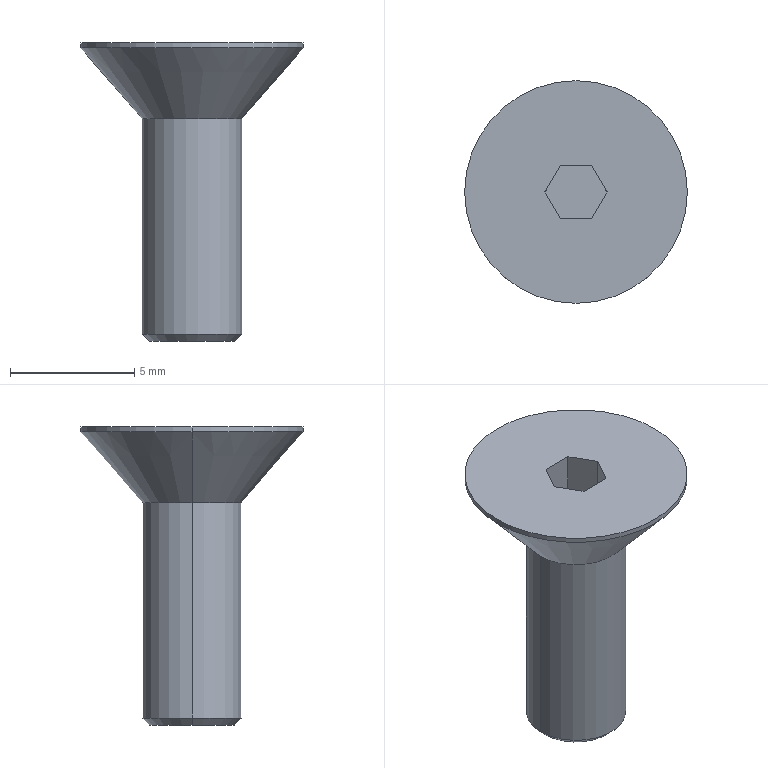Part | STEP file | 4-20.sldasm-Part-284 | 1 solid | 17 faces | box 8.96 x 8.96 x 12 mm | volume 213.091 mm3 | plane 9 | cone 4 | cylinder 4 | commonest cylinder face diameters 4 x2 8.96 x2
STEP:
#1=CARTESIAN_POINT('',(1.716,545.,-147.5));
#2=VERTEX_POINT('',#1);
#3=CARTESIAN_POINT('',(-1.716,545.,-147.5));
#4=VERTEX_POINT('',#3);
#5=CARTESIAN_POINT('',(0.,545.,-147.5));
#6=DIRECTION('',(0.,0.,-1.));
#7=DIRECTION('',(1.,0.,0.));
#8=AXIS2_PLACEMENT_3D('',#5,#6,#7);
#9=CIRCLE('',#8,1.716);
#10=EDGE_CURVE('',#2,#4,#9,.T.);
#11=ORIENTED_EDGE('',*,*,#10,.F.);
#12=CARTESIAN_POINT('',(2.,545.,-147.216));
#13=VERTEX_POINT('',#12);
#14=CARTESIAN_POINT('',(2.,545.,-147.216));
#15=DIRECTION('',(0.7071,0.,0.7071));
#16=VECTOR('',#15,1000.);
#17=LINE('',#14,#16);
#18=EDGE_CURVE('',#2,#13,#17,.T.);
#19=ORIENTED_EDGE('',*,*,#18,.T.);
#20=CARTESIAN_POINT('',(-2.,545.,-147.216));
#21=VERTEX_POINT('',#20);
#22=CARTESIAN_POINT('',(0.,545.,-147.216));
#23=DIRECTION('',(0.,0.,1.));
#24=DIRECTION('',(1.,0.,0.));
#25=AXIS2_PLACEMENT_3D('',#22,#23,#24);
#26=CIRCLE('',#25,2.);
#27=EDGE_CURVE('',#21,#13,#26,.T.);
#28=ORIENTED_EDGE('',*,*,#27,.F.);
#29=CARTESIAN_POINT('',(-2.,545.,-147.216));
#30=DIRECTION('',(-0.7071,0.,0.7071));
#31=VECTOR('',#30,1000.);
#32=LINE('',#29,#31);
#33=EDGE_CURVE('',#4,#21,#32,.T.);
#34=ORIENTED_EDGE('',*,*,#33,.F.);
#35=EDGE_LOOP('',(#11,#19,#28,#34));
#36=FACE_OUTER_BOUND('',#35,.T.);
#37=CARTESIAN_POINT('',(0.,545.,-147.216));
#38=DIRECTION('',(0.,0.,1.));
#39=DIRECTION('',(-1.,0.,0.));
#40=AXIS2_PLACEMENT_3D('',#37,#38,#39);
#41=CONICAL_SURFACE('',#40,2.,0.7854);
#42=ADVANCED_FACE('',(#36),#41,.T.);
#43=ORIENTED_EDGE('',*,*,#27,.T.);
#44=CARTESIAN_POINT('',(2.,545.,-138.553));
#45=VERTEX_POINT('',#44);
#46=CARTESIAN_POINT('',(2.,545.,-135.));
#47=DIRECTION('',(0.,0.,1.));
#48=VECTOR('',#47,1000.);
#49=LINE('',#46,#48);
#50=EDGE_CURVE('',#13,#45,#49,.T.);
#51=ORIENTED_EDGE('',*,*,#50,.T.);
#52=CARTESIAN_POINT('',(-2.,545.,-138.553));
#53=VERTEX_POINT('',#52);
#54=CARTESIAN_POINT('',(0.,545.,-138.553));
#55=DIRECTION('',(0.,0.,1.));
#56=DIRECTION('',(-1.,0.,0.));
#57=AXIS2_PLACEMENT_3D('',#54,#55,#56);
#58=CIRCLE('',#57,2.);
#59=EDGE_CURVE('',#53,#45,#58,.T.);
#60=ORIENTED_EDGE('',*,*,#59,.F.);
#61=CARTESIAN_POINT('',(-2.,545.,-135.));
#62=DIRECTION('',(0.,0.,1.));
#63=VECTOR('',#62,1000.);
#64=LINE('',#61,#63);
#65=EDGE_CURVE('',#21,#53,#64,.T.);
#66=ORIENTED_EDGE('',*,*,#65,.F.);
#67=EDGE_LOOP('',(#43,#51,#60,#66));
#68=FACE_OUTER_BOUND('',#67,.T.);
#69=CARTESIAN_POINT('',(0.,545.,-135.));
#70=DIRECTION('',(0.,0.,1.));
#71=DIRECTION('',(-1.,0.,0.));
#72=AXIS2_PLACEMENT_3D('',#69,#70,#71);
#73=CYLINDRICAL_SURFACE('',#72,2.);
#74=ADVANCED_FACE('',(#68),#73,.T.);
#75=ORIENTED_EDGE('',*,*,#59,.T.);
#76=CARTESIAN_POINT('',(4.48,545.,-135.7));
#77=VERTEX_POINT('',#76);
#78=CARTESIAN_POINT('',(4.48,545.,-135.7));
#79=DIRECTION('',(0.6561,0.,0.7547));
#80=VECTOR('',#79,1000.);
#81=LINE('',#78,#80);
#82=EDGE_CURVE('',#45,#77,#81,.T.);
#83=ORIENTED_EDGE('',*,*,#82,.T.);
#84=CARTESIAN_POINT('',(-4.48,545.,-135.7));
#85=VERTEX_POINT('',#84);
#86=CARTESIAN_POINT('',(0.,545.,-135.7));
#87=DIRECTION('',(0.,0.,1.));
#88=DIRECTION('',(-1.,0.,0.));
#89=AXIS2_PLACEMENT_3D('',#86,#87,#88);
#90=CIRCLE('',#89,4.48);
#91=EDGE_CURVE('',#85,#77,#90,.T.);
#92=ORIENTED_EDGE('',*,*,#91,.F.);
#93=CARTESIAN_POINT('',(-4.48,545.,-135.7));
#94=DIRECTION('',(-0.6561,0.,0.7547));
#95=VECTOR('',#94,1000.);
#96=LINE('',#93,#95);
#97=EDGE_CURVE('',#53,#85,#96,.T.);
#98=ORIENTED_EDGE('',*,*,#97,.F.);
#99=EDGE_LOOP('',(#75,#83,#92,#98));
#100=FACE_OUTER_BOUND('',#99,.T.);
#101=CARTESIAN_POINT('',(0.,545.,-135.7));
#102=DIRECTION('',(0.,0.,1.));
#103=DIRECTION('',(-1.,0.,0.));
#104=AXIS2_PLACEMENT_3D('',#101,#102,#103);
#105=CONICAL_SURFACE('',#104,4.48,0.7156);
#106=ADVANCED_FACE('',(#100),#105,.T.);
#107=ORIENTED_EDGE('',*,*,#91,.T.);
#108=CARTESIAN_POINT('',(4.48,545.,-135.5));
#109=VERTEX_POINT('',#108);
#110=CARTESIAN_POINT('',(4.48,545.,-135.));
#111=DIRECTION('',(0.,0.,1.));
#112=VECTOR('',#111,1000.);
#113=LINE('',#110,#112);
#114=EDGE_CURVE('',#77,#109,#113,.T.);
#115=ORIENTED_EDGE('',*,*,#114,.T.);
#116=CARTESIAN_POINT('',(-4.48,545.,-135.5));
#117=VERTEX_POINT('',#116);
#118=CARTESIAN_POINT('',(0.,545.,-135.5));
#119=DIRECTION('',(0.,0.,1.));
#120=DIRECTION('',(-1.,0.,0.));
#121=AXIS2_PLACEMENT_3D('',#118,#119,#120);
#122=CIRCLE('',#121,4.48);
#123=EDGE_CURVE('',#117,#109,#122,.T.);
#124=ORIENTED_EDGE('',*,*,#123,.F.);
#125=CARTESIAN_POINT('',(-4.48,545.,-135.));
#126=DIRECTION('',(0.,0.,1.));
#127=VECTOR('',#126,1000.);
#128=LINE('',#125,#127);
#129=EDGE_CURVE('',#85,#117,#128,.T.);
#130=ORIENTED_EDGE('',*,*,#129,.F.);
#131=EDGE_LOOP('',(#107,#115,#124,#130));
#132=FACE_OUTER_BOUND('',#131,.T.);
#133=CARTESIAN_POINT('',(0.,545.,-135.));
#134=DIRECTION('',(0.,0.,1.));
#135=DIRECTION('',(-1.,0.,0.));
#136=AXIS2_PLACEMENT_3D('',#133,#134,#135);
#137=CYLINDRICAL_SURFACE('',#136,4.48);
#138=ADVANCED_FACE('',(#132),#137,.T.);
#139=CARTESIAN_POINT('',(0.,545.,-147.5));
#140=DIRECTION('',(0.,0.,-1.));
#141=DIRECTION('',(1.,0.,0.));
#142=AXIS2_PLACEMENT_3D('',#139,#140,#141);
#143=CIRCLE('',#142,1.716);
#144=EDGE_CURVE('',#4,#2,#143,.T.);
#145=ORIENTED_EDGE('',*,*,#144,.T.);
#146=ORIENTED_EDGE('',*,*,#10,.T.);
#147=EDGE_LOOP('',(#145,#146));
#148=FACE_OUTER_BOUND('',#147,.T.);
#149=CARTESIAN_POINT('',(-2.,545.,-147.5));
#150=DIRECTION('',(0.,0.,-1.));
#151=DIRECTION('',(1.,0.,0.));
#152=AXIS2_PLACEMENT_3D('',#149,#150,#151);
#153=PLANE('',#152);
#154=ADVANCED_FACE('',(#148),#153,.T.);
#155=ORIENTED_EDGE('',*,*,#50,.F.);
#156=CARTESIAN_POINT('',(0.,545.,-147.216));
#157=DIRECTION('',(0.,0.,1.));
#158=DIRECTION('',(1.,0.,0.));
#159=AXIS2_PLACEMENT_3D('',#156,#157,#158);
#160=CIRCLE('',#159,2.);
#161=EDGE_CURVE('',#13,#21,#160,.T.);
#162=ORIENTED_EDGE('',*,*,#161,.T.);
#163=ORIENTED_EDGE('',*,*,#65,.T.);
#164=CARTESIAN_POINT('',(0.,545.,-138.553));
#165=DIRECTION('',(0.,0.,1.));
#166=DIRECTION('',(-1.,0.,0.));
#167=AXIS2_PLACEMENT_3D('',#164,#165,#166);
#168=CIRCLE('',#167,2.);
#169=EDGE_CURVE('',#45,#53,#168,.T.);
#170=ORIENTED_EDGE('',*,*,#169,.F.);
#171=EDGE_LOOP('',(#155,#162,#163,#170));
#172=FACE_OUTER_BOUND('',#171,.T.);
#173=CARTESIAN_POINT('',(0.,545.,-135.));
#174=DIRECTION('',(0.,0.,1.));
#175=DIRECTION('',(-1.,0.,0.));
#176=AXIS2_PLACEMENT_3D('',#173,#174,#175);
#177=CYLINDRICAL_SURFACE('',#176,2.);
#178=ADVANCED_FACE('',(#172),#177,.T.);
#179=ORIENTED_EDGE('',*,*,#82,.F.);
#180=ORIENTED_EDGE('',*,*,#169,.T.);
#181=ORIENTED_EDGE('',*,*,#97,.T.);
#182=CARTESIAN_POINT('',(0.,545.,-135.7));
#183=DIRECTION('',(0.,0.,1.));
#184=DIRECTION('',(-1.,0.,0.));
#185=AXIS2_PLACEMENT_3D('',#182,#183,#184);
#186=CIRCLE('',#185,4.48);
#187=EDGE_CURVE('',#77,#85,#186,.T.);
#188=ORIENTED_EDGE('',*,*,#187,.F.);
#189=EDGE_LOOP('',(#179,#180,#181,#188));
#190=FACE_OUTER_BOUND('',#189,.T.);
#191=CARTESIAN_POINT('',(0.,545.,-135.7));
#192=DIRECTION('',(0.,0.,1.));
#193=DIRECTION('',(-1.,0.,0.));
#194=AXIS2_PLACEMENT_3D('',#191,#192,#193);
#195=CONICAL_SURFACE('',#194,4.48,0.7156);
#196=ADVANCED_FACE('',(#190),#195,.T.);
#197=ORIENTED_EDGE('',*,*,#114,.F.);
#198=ORIENTED_EDGE('',*,*,#187,.T.);
#199=ORIENTED_EDGE('',*,*,#129,.T.);
#200=CARTESIAN_POINT('',(0.,545.,-135.5));
#201=DIRECTION('',(0.,0.,1.));
#202=DIRECTION('',(-1.,0.,0.));
#203=AXIS2_PLACEMENT_3D('',#200,#201,#202);
#204=CIRCLE('',#203,4.48);
#205=EDGE_CURVE('',#109,#117,#204,.T.);
#206=ORIENTED_EDGE('',*,*,#205,.F.);
#207=EDGE_LOOP('',(#197,#198,#199,#206));
#208=FACE_OUTER_BOUND('',#207,.T.);
#209=CARTESIAN_POINT('',(0.,545.,-135.));
#210=DIRECTION('',(0.,0.,1.));
#211=DIRECTION('',(-1.,0.,0.));
#212=AXIS2_PLACEMENT_3D('',#209,#210,#211);
#213=CYLINDRICAL_SURFACE('',#212,4.48);
#214=ADVANCED_FACE('',(#208),#213,.T.);
#215=CARTESIAN_POINT('',(-0.625,543.917,-135.5));
#216=VERTEX_POINT('',#215);
#217=CARTESIAN_POINT('',(0.625,543.917,-135.5));
#218=VERTEX_POINT('',#217);
#219=CARTESIAN_POINT('',(-0.625,543.917,-135.5));
#220=DIRECTION('',(1.,0.,0.));
#221=VECTOR('',#220,1000.);
#222=LINE('',#219,#221);
#223=EDGE_CURVE('',#216,#218,#222,.T.);
#224=ORIENTED_EDGE('',*,*,#223,.F.);
#225=CARTESIAN_POINT('',(-1.25,545.,-135.5));
#226=VERTEX_POINT('',#225);
#227=CARTESIAN_POINT('',(-1.25,545.,-135.5));
#228=DIRECTION('',(0.5,-0.866,0.));
#229=VECTOR('',#228,1000.);
#230=LINE('',#227,#229);
#231=EDGE_CURVE('',#226,#216,#230,.T.);
#232=ORIENTED_EDGE('',*,*,#231,.F.);
#233=CARTESIAN_POINT('',(-0.625,546.083,-135.5));
#234=VERTEX_POINT('',#233);
#235=CARTESIAN_POINT('',(-0.625,546.083,-135.5));
#236=DIRECTION('',(-0.5,-0.866,0.));
#237=VECTOR('',#236,1000.);
#238=LINE('',#235,#237);
#239=EDGE_CURVE('',#234,#226,#238,.T.);
#240=ORIENTED_EDGE('',*,*,#239,.F.);
#241=CARTESIAN_POINT('',(0.625,546.083,-135.5));
#242=VERTEX_POINT('',#241);
#243=CARTESIAN_POINT('',(0.625,546.083,-135.5));
#244=DIRECTION('',(-1.,0.,0.));
#245=VECTOR('',#244,1000.);
#246=LINE('',#243,#245);
#247=EDGE_CURVE('',#242,#234,#246,.T.);
#248=ORIENTED_EDGE('',*,*,#247,.F.);
#249=CARTESIAN_POINT('',(1.25,545.,-135.5));
#250=VERTEX_POINT('',#249);
#251=CARTESIAN_POINT('',(1.25,545.,-135.5));
#252=DIRECTION('',(-0.5,0.866,0.));
#253=VECTOR('',#252,1000.);
#254=LINE('',#251,#253);
#255=EDGE_CURVE('',#250,#242,#254,.T.);
#256=ORIENTED_EDGE('',*,*,#255,.F.);
#257=CARTESIAN_POINT('',(0.625,543.917,-135.5));
#258=DIRECTION('',(0.5,0.866,0.));
#259=VECTOR('',#258,1000.);
#260=LINE('',#257,#259);
#261=EDGE_CURVE('',#218,#250,#260,.T.);
#262=ORIENTED_EDGE('',*,*,#261,.F.);
#263=EDGE_LOOP('',(#224,#232,#240,#248,#256,#262));
#264=FACE_BOUND('',#263,.T.);
#265=ORIENTED_EDGE('',*,*,#123,.T.);
#266=ORIENTED_EDGE('',*,*,#205,.T.);
#267=EDGE_LOOP('',(#265,#266));
#268=FACE_OUTER_BOUND('',#267,.T.);
#269=CARTESIAN_POINT('',(0.,545.,-135.5));
#270=DIRECTION('',(0.,0.,1.));
#271=DIRECTION('',(-1.,0.,0.));
#272=AXIS2_PLACEMENT_3D('',#269,#270,#271);
#273=PLANE('',#272);
#274=ADVANCED_FACE('',(#264,#268),#273,.T.);
#275=ORIENTED_EDGE('',*,*,#18,.F.);
#276=ORIENTED_EDGE('',*,*,#144,.F.);
#277=ORIENTED_EDGE('',*,*,#33,.T.);
#278=ORIENTED_EDGE('',*,*,#161,.F.);
#279=EDGE_LOOP('',(#275,#276,#277,#278));
#280=FACE_OUTER_BOUND('',#279,.T.);
#281=CARTESIAN_POINT('',(0.,545.,-147.216));
#282=DIRECTION('',(0.,0.,1.));
#283=DIRECTION('',(-1.,0.,0.));
#284=AXIS2_PLACEMENT_3D('',#281,#282,#283);
#285=CONICAL_SURFACE('',#284,2.,0.7854);
#286=ADVANCED_FACE('',(#280),#285,.T.);
#287=ORIENTED_EDGE('',*,*,#223,.T.);
#288=CARTESIAN_POINT('',(0.625,543.917,-138.));
#289=VERTEX_POINT('',#288);
#290=CARTESIAN_POINT('',(0.625,543.917,-138.));
#291=DIRECTION('',(0.,0.,1.));
#292=VECTOR('',#291,1000.);
#293=LINE('',#290,#292);
#294=EDGE_CURVE('',#289,#218,#293,.T.);
#295=ORIENTED_EDGE('',*,*,#294,.F.);
#296=CARTESIAN_POINT('',(-0.625,543.917,-138.));
#297=VERTEX_POINT('',#296);
#298=CARTESIAN_POINT('',(-0.625,543.917,-138.));
#299=DIRECTION('',(1.,0.,0.));
#300=VECTOR('',#299,1000.);
#301=LINE('',#298,#300);
#302=EDGE_CURVE('',#297,#289,#301,.T.);
#303=ORIENTED_EDGE('',*,*,#302,.F.);
#304=CARTESIAN_POINT('',(-0.625,543.917,-138.));
#305=DIRECTION('',(0.,0.,1.));
#306=VECTOR('',#305,1000.);
#307=LINE('',#304,#306);
#308=EDGE_CURVE('',#297,#216,#307,.T.);
#309=ORIENTED_EDGE('',*,*,#308,.T.);
#310=EDGE_LOOP('',(#287,#295,#303,#309));
#311=FACE_OUTER_BOUND('',#310,.T.);
#312=CARTESIAN_POINT('',(-0.625,543.917,-138.));
#313=DIRECTION('',(0.,-1.,0.));
#314=DIRECTION('',(0.,0.,1.));
#315=AXIS2_PLACEMENT_3D('',#312,#313,#314);
#316=PLANE('',#315);
#317=ADVANCED_FACE('',(#311),#316,.F.);
#318=ORIENTED_EDGE('',*,*,#261,.T.);
#319=CARTESIAN_POINT('',(1.25,545.,-138.));
#320=VERTEX_POINT('',#319);
#321=CARTESIAN_POINT('',(1.25,545.,-138.));
#322=DIRECTION('',(0.,0.,1.));
#323=VECTOR('',#322,1000.);
#324=LINE('',#321,#323);
#325=EDGE_CURVE('',#320,#250,#324,.T.);
#326=ORIENTED_EDGE('',*,*,#325,.F.);
#327=CARTESIAN_POINT('',(0.625,543.917,-138.));
#328=DIRECTION('',(0.5,0.866,0.));
#329=VECTOR('',#328,1000.);
#330=LINE('',#327,#329);
#331=EDGE_CURVE('',#289,#320,#330,.T.);
#332=ORIENTED_EDGE('',*,*,#331,.F.);
#333=ORIENTED_EDGE('',*,*,#294,.T.);
#334=EDGE_LOOP('',(#318,#326,#332,#333));
#335=FACE_OUTER_BOUND('',#334,.T.);
#336=CARTESIAN_POINT('',(0.625,543.917,-138.));
#337=DIRECTION('',(0.866,-0.5,0.));
#338=DIRECTION('',(0.5,0.866,0.));
#339=AXIS2_PLACEMENT_3D('',#336,#337,#338);
#340=PLANE('',#339);
#341=ADVANCED_FACE('',(#335),#340,.F.);
#342=ORIENTED_EDGE('',*,*,#255,.T.);
#343=CARTESIAN_POINT('',(0.625,546.083,-138.));
#344=VERTEX_POINT('',#343);
#345=CARTESIAN_POINT('',(0.625,546.083,-138.));
#346=DIRECTION('',(0.,0.,1.));
#347=VECTOR('',#346,1000.);
#348=LINE('',#345,#347);
#349=EDGE_CURVE('',#344,#242,#348,.T.);
#350=ORIENTED_EDGE('',*,*,#349,.F.);
#351=CARTESIAN_POINT('',(1.25,545.,-138.));
#352=DIRECTION('',(-0.5,0.866,0.));
#353=VECTOR('',#352,1000.);
#354=LINE('',#351,#353);
#355=EDGE_CURVE('',#320,#344,#354,.T.);
#356=ORIENTED_EDGE('',*,*,#355,.F.);
#357=ORIENTED_EDGE('',*,*,#325,.T.);
#358=EDGE_LOOP('',(#342,#350,#356,#357));
#359=FACE_OUTER_BOUND('',#358,.T.);
#360=CARTESIAN_POINT('',(1.25,545.,-138.));
#361=DIRECTION('',(0.866,0.5,0.));
#362=DIRECTION('',(-0.5,0.866,0.));
#363=AXIS2_PLACEMENT_3D('',#360,#361,#362);
#364=PLANE('',#363);
#365=ADVANCED_FACE('',(#359),#364,.F.);
#366=ORIENTED_EDGE('',*,*,#247,.T.);
#367=CARTESIAN_POINT('',(-0.625,546.083,-138.));
#368=VERTEX_POINT('',#367);
#369=CARTESIAN_POINT('',(-0.625,546.083,-138.));
#370=DIRECTION('',(0.,0.,1.));
#371=VECTOR('',#370,1000.);
#372=LINE('',#369,#371);
#373=EDGE_CURVE('',#368,#234,#372,.T.);
#374=ORIENTED_EDGE('',*,*,#373,.F.);
#375=CARTESIAN_POINT('',(0.625,546.083,-138.));
#376=DIRECTION('',(-1.,0.,0.));
#377=VECTOR('',#376,1000.);
#378=LINE('',#375,#377);
#379=EDGE_CURVE('',#344,#368,#378,.T.);
#380=ORIENTED_EDGE('',*,*,#379,.F.);
#381=ORIENTED_EDGE('',*,*,#349,.T.);
#382=EDGE_LOOP('',(#366,#374,#380,#381));
#383=FACE_OUTER_BOUND('',#382,.T.);
#384=CARTESIAN_POINT('',(0.625,546.083,-138.));
#385=DIRECTION('',(0.,1.,0.));
#386=DIRECTION('',(0.,0.,-1.));
#387=AXIS2_PLACEMENT_3D('',#384,#385,#386);
#388=PLANE('',#387);
#389=ADVANCED_FACE('',(#383),#388,.F.);
#390=ORIENTED_EDGE('',*,*,#239,.T.);
#391=CARTESIAN_POINT('',(-1.25,545.,-138.));
#392=VERTEX_POINT('',#391);
#393=CARTESIAN_POINT('',(-1.25,545.,-138.));
#394=DIRECTION('',(0.,0.,1.));
#395=VECTOR('',#394,1000.);
#396=LINE('',#393,#395);
#397=EDGE_CURVE('',#392,#226,#396,.T.);
#398=ORIENTED_EDGE('',*,*,#397,.F.);
#399=CARTESIAN_POINT('',(-0.625,546.083,-138.));
#400=DIRECTION('',(-0.5,-0.866,0.));
#401=VECTOR('',#400,1000.);
#402=LINE('',#399,#401);
#403=EDGE_CURVE('',#368,#392,#402,.T.);
#404=ORIENTED_EDGE('',*,*,#403,.F.);
#405=ORIENTED_EDGE('',*,*,#373,.T.);
#406=EDGE_LOOP('',(#390,#398,#404,#405));
#407=FACE_OUTER_BOUND('',#406,.T.);
#408=CARTESIAN_POINT('',(-0.625,546.083,-138.));
#409=DIRECTION('',(-0.866,0.5,0.));
#410=DIRECTION('',(-0.5,-0.866,0.));
#411=AXIS2_PLACEMENT_3D('',#408,#409,#410);
#412=PLANE('',#411);
#413=ADVANCED_FACE('',(#407),#412,.F.);
#414=ORIENTED_EDGE('',*,*,#231,.T.);
#415=ORIENTED_EDGE('',*,*,#308,.F.);
#416=CARTESIAN_POINT('',(-1.25,545.,-138.));
#417=DIRECTION('',(0.5,-0.866,0.));
#418=VECTOR('',#417,1000.);
#419=LINE('',#416,#418);
#420=EDGE_CURVE('',#392,#297,#419,.T.);
#421=ORIENTED_EDGE('',*,*,#420,.F.);
#422=ORIENTED_EDGE('',*,*,#397,.T.);
#423=EDGE_LOOP('',(#414,#415,#421,#422));
#424=FACE_OUTER_BOUND('',#423,.T.);
#425=CARTESIAN_POINT('',(-1.25,545.,-138.));
#426=DIRECTION('',(-0.866,-0.5,0.));
#427=DIRECTION('',(0.5,-0.866,0.));
#428=AXIS2_PLACEMENT_3D('',#425,#426,#427);
#429=PLANE('',#428);
#430=ADVANCED_FACE('',(#424),#429,.F.);
#431=ORIENTED_EDGE('',*,*,#302,.T.);
#432=ORIENTED_EDGE('',*,*,#331,.T.);
#433=ORIENTED_EDGE('',*,*,#355,.T.);
#434=ORIENTED_EDGE('',*,*,#379,.T.);
#435=ORIENTED_EDGE('',*,*,#403,.T.);
#436=ORIENTED_EDGE('',*,*,#420,.T.);
#437=EDGE_LOOP('',(#431,#432,#433,#434,#435,#436));
#438=FACE_OUTER_BOUND('',#437,.T.);
#439=CARTESIAN_POINT('',(0.625,543.917,-138.));
#440=DIRECTION('',(0.,0.,1.));
#441=DIRECTION('',(0.,1.,0.));
#442=AXIS2_PLACEMENT_3D('',#439,#440,#441);
#443=PLANE('',#442);
#444=ADVANCED_FACE('',(#438),#443,.T.);
#445=CLOSED_SHELL('',(#42,#74,#106,#138,#154,#178,#196,#214,#274,#286,#317,#341,#365,#389,#413,#430,#444));
#446=MANIFOLD_SOLID_BREP('',#445);
#447=CARTESIAN_POINT('',(0.,0.,0.));
#448=DIRECTION('',(0.,0.,1.));
#449=DIRECTION('',(1.,0.,0.));
#450=AXIS2_PLACEMENT_3D('',#447,#448,#449);
#451=(LENGTH_UNIT()NAMED_UNIT(*)SI_UNIT(.MILLI.,.METRE.));
#452=UNCERTAINTY_MEASURE_WITH_UNIT(LENGTH_MEASURE(0.00001),#451,'','');
#453=(NAMED_UNIT(*)PLANE_ANGLE_UNIT()SI_UNIT($,.RADIAN.));
#454=(NAMED_UNIT(*)SI_UNIT($,.STERADIAN.)SOLID_ANGLE_UNIT());
#455=(GEOMETRIC_REPRESENTATION_CONTEXT(3)GLOBAL_UNCERTAINTY_ASSIGNED_CONTEXT((#452))GLOBAL_UNIT_ASSIGNED_CONTEXT((#451,#453,#454))REPRESENTATION_CONTEXT('',''));
#456=ADVANCED_BREP_SHAPE_REPRESENTATION('',(#446,#450),#455);